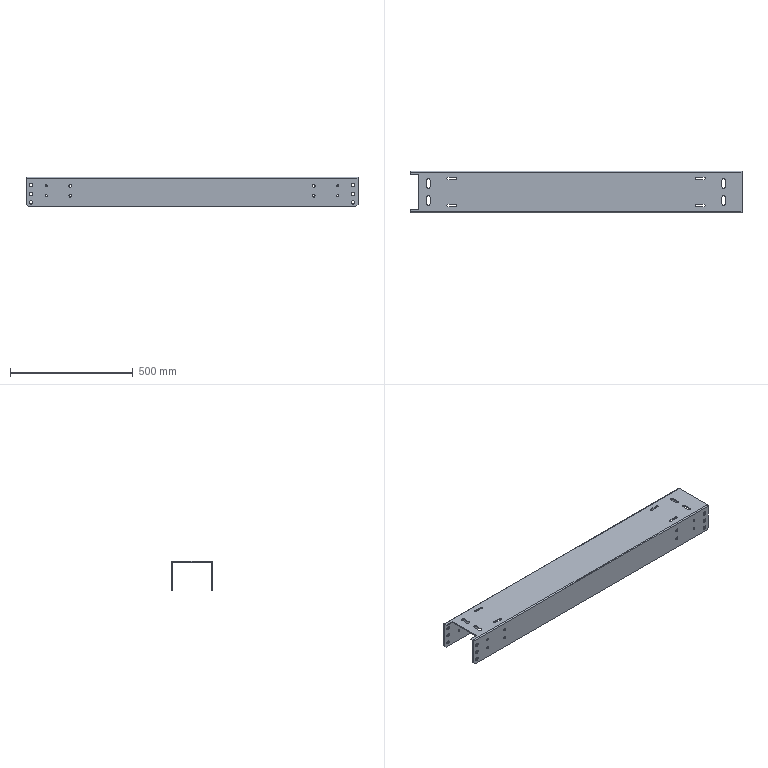Part | SolidWorks | features ICE 2, Chamfer 1, FlatPattern 1, SMBaseFlange 1, SheetMetal 1 | 1 solid | 122 faces | box 1350 x 170 x 120 mm | volume 2114515 mm3 | cylinder 80 | plane 42 | commonest cylinder face diameters 9 x28 14 x24 11 x16 13 x8 0.4 x2 8.4 x2